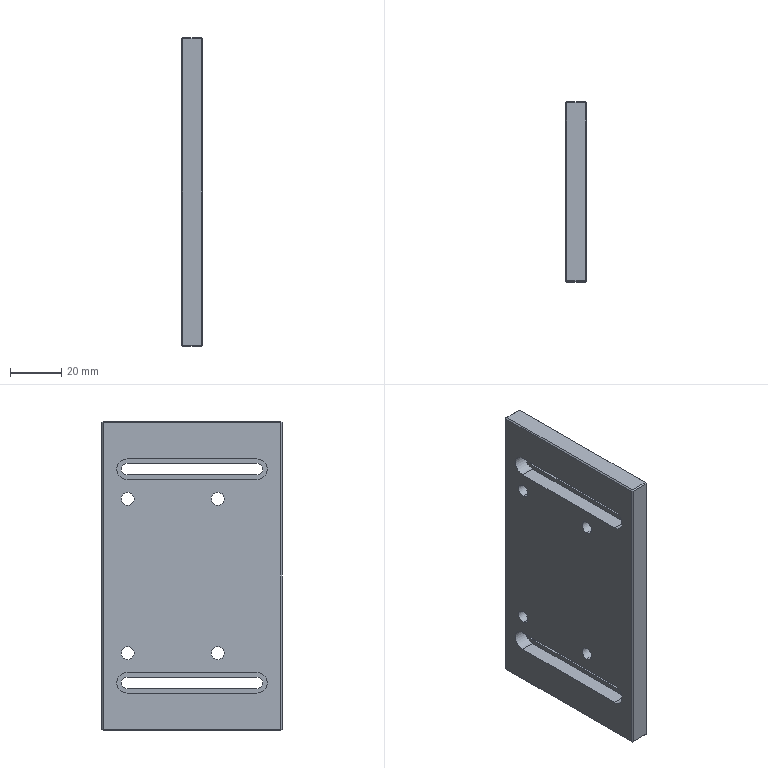Part | SolidWorks | features HoleWzd 3, Chamfer 2, Extrusion 1, ICE 1 | 1 solid | 64 faces | box 8 x 70 x 120 mm | volume 59993 mm3 | plane 36 | cylinder 22 | cone 6 | commonest cylinder face diameters 5 x8 3.3 x6 4.5 x4 8 x4